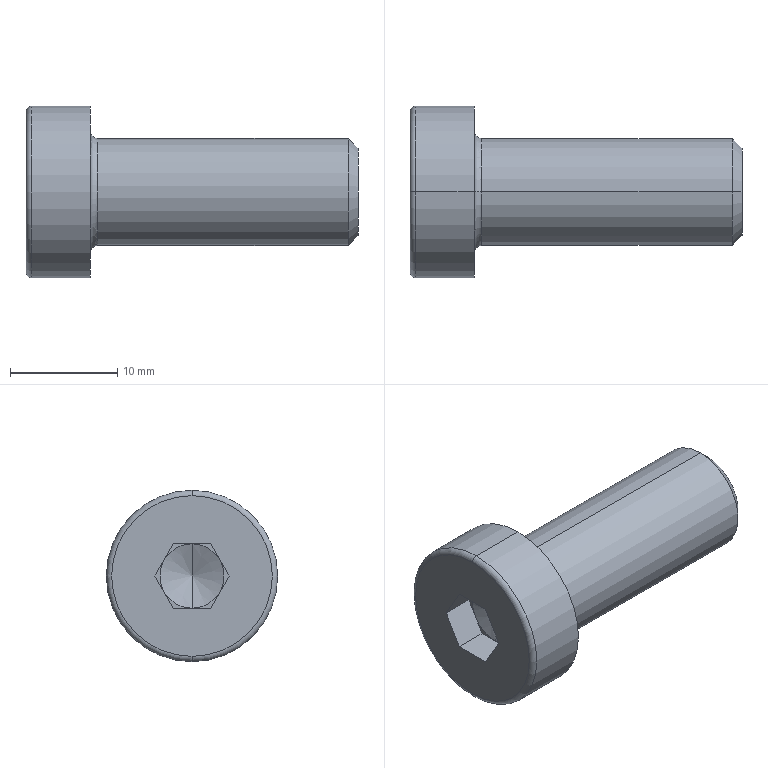Part | STEP file | 1 solid | 27 faces | box 31 x 16 x 16 mm | volume 3053 mm3 | plane 15 | cone 4 | cylinder 4 | torus 4 | commonest cylinder face diameters 10 x2 16 x2